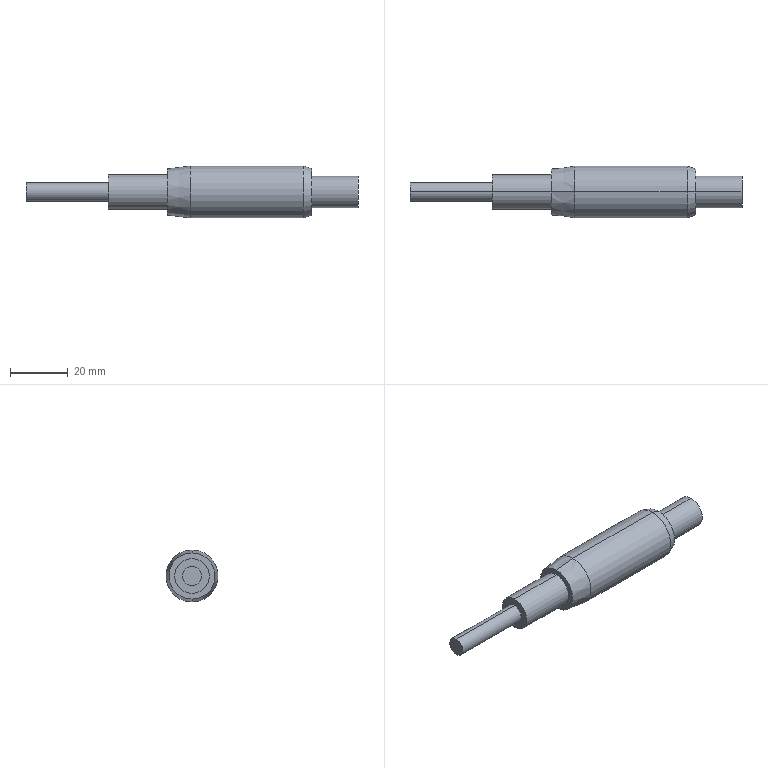Part | SolidWorks | features Revolution 1 | 1 solid | 17 faces | box 115 x 18 x 18 mm | volume 17209 mm3 | cylinder 8 | plane 5 | cone 4 | commonest cylinder face diameters 6.5 x2 11 x2 12 x2 18 x2
STEP:
#1=CARTESIAN_POINT('',(0.,0.,-3.25));
#2=VERTEX_POINT('',#1);
#3=CARTESIAN_POINT('',(0.,0.,3.25));
#4=VERTEX_POINT('',#3);
#5=CARTESIAN_POINT('',(0.,0.,0.));
#6=DIRECTION('',(1.,0.,0.));
#7=DIRECTION('',(0.,0.,-1.));
#8=AXIS2_PLACEMENT_3D('',#5,#6,#7);
#9=CIRCLE('',#8,3.25);
#10=EDGE_CURVE('',#2,#4,#9,.T.);
#11=ORIENTED_EDGE('',*,*,#10,.T.);
#12=CARTESIAN_POINT('',(28.5,0.,3.25));
#13=VERTEX_POINT('',#12);
#14=CARTESIAN_POINT('',(115.,0.,3.25));
#15=DIRECTION('',(1.,0.,0.));
#16=VECTOR('',#15,1000.);
#17=LINE('',#14,#16);
#18=EDGE_CURVE('',#4,#13,#17,.T.);
#19=ORIENTED_EDGE('',*,*,#18,.T.);
#20=CARTESIAN_POINT('',(28.5,0.,-3.25));
#21=VERTEX_POINT('',#20);
#22=CARTESIAN_POINT('',(28.5,0.,0.));
#23=DIRECTION('',(1.,0.,0.));
#24=DIRECTION('',(0.,0.,-1.));
#25=AXIS2_PLACEMENT_3D('',#22,#23,#24);
#26=CIRCLE('',#25,3.25);
#27=EDGE_CURVE('',#21,#13,#26,.T.);
#28=ORIENTED_EDGE('',*,*,#27,.F.);
#29=CARTESIAN_POINT('',(115.,0.,-3.25));
#30=DIRECTION('',(1.,0.,0.));
#31=VECTOR('',#30,1000.);
#32=LINE('',#29,#31);
#33=EDGE_CURVE('',#2,#21,#32,.T.);
#34=ORIENTED_EDGE('',*,*,#33,.F.);
#35=EDGE_LOOP('',(#11,#19,#28,#34));
#36=FACE_OUTER_BOUND('',#35,.T.);
#37=CARTESIAN_POINT('',(115.,0.,0.));
#38=DIRECTION('',(1.,0.,0.));
#39=DIRECTION('',(0.,0.,-1.));
#40=AXIS2_PLACEMENT_3D('',#37,#38,#39);
#41=CYLINDRICAL_SURFACE('',#40,3.25);
#42=ADVANCED_FACE('',(#36),#41,.T.);
#43=CARTESIAN_POINT('',(99.,0.,-5.5));
#44=VERTEX_POINT('',#43);
#45=CARTESIAN_POINT('',(99.,0.,5.5));
#46=VERTEX_POINT('',#45);
#47=CARTESIAN_POINT('',(99.,0.,0.));
#48=DIRECTION('',(1.,0.,0.));
#49=DIRECTION('',(0.,0.,-1.));
#50=AXIS2_PLACEMENT_3D('',#47,#48,#49);
#51=CIRCLE('',#50,5.5);
#52=EDGE_CURVE('',#44,#46,#51,.T.);
#53=ORIENTED_EDGE('',*,*,#52,.T.);
#54=CARTESIAN_POINT('',(115.,0.,5.5));
#55=VERTEX_POINT('',#54);
#56=CARTESIAN_POINT('',(115.,0.,5.5));
#57=DIRECTION('',(1.,0.,0.));
#58=VECTOR('',#57,1000.);
#59=LINE('',#56,#58);
#60=EDGE_CURVE('',#46,#55,#59,.T.);
#61=ORIENTED_EDGE('',*,*,#60,.T.);
#62=CARTESIAN_POINT('',(115.,0.,-5.5));
#63=VERTEX_POINT('',#62);
#64=CARTESIAN_POINT('',(115.,0.,0.));
#65=DIRECTION('',(1.,0.,0.));
#66=DIRECTION('',(0.,0.,-1.));
#67=AXIS2_PLACEMENT_3D('',#64,#65,#66);
#68=CIRCLE('',#67,5.5);
#69=EDGE_CURVE('',#63,#55,#68,.T.);
#70=ORIENTED_EDGE('',*,*,#69,.F.);
#71=CARTESIAN_POINT('',(115.,0.,-5.5));
#72=DIRECTION('',(1.,0.,0.));
#73=VECTOR('',#72,1000.);
#74=LINE('',#71,#73);
#75=EDGE_CURVE('',#44,#63,#74,.T.);
#76=ORIENTED_EDGE('',*,*,#75,.F.);
#77=EDGE_LOOP('',(#53,#61,#70,#76));
#78=FACE_OUTER_BOUND('',#77,.T.);
#79=CARTESIAN_POINT('',(115.,0.,0.));
#80=DIRECTION('',(1.,0.,0.));
#81=DIRECTION('',(0.,0.,-1.));
#82=AXIS2_PLACEMENT_3D('',#79,#80,#81);
#83=CYLINDRICAL_SURFACE('',#82,5.5);
#84=ADVANCED_FACE('',(#78),#83,.T.);
#85=CARTESIAN_POINT('',(99.,0.,-8.));
#86=VERTEX_POINT('',#85);
#87=CARTESIAN_POINT('',(99.,0.,8.));
#88=VERTEX_POINT('',#87);
#89=CARTESIAN_POINT('',(99.,0.,0.));
#90=DIRECTION('',(1.,0.,0.));
#91=DIRECTION('',(0.,0.,-1.));
#92=AXIS2_PLACEMENT_3D('',#89,#90,#91);
#93=CIRCLE('',#92,8.);
#94=EDGE_CURVE('',#86,#88,#93,.T.);
#95=ORIENTED_EDGE('',*,*,#94,.F.);
#96=CARTESIAN_POINT('',(96.,0.,-9.));
#97=VERTEX_POINT('',#96);
#98=CARTESIAN_POINT('',(99.,0.,-8.));
#99=DIRECTION('',(-0.9487,0.,-0.3162));
#100=VECTOR('',#99,1000.);
#101=LINE('',#98,#100);
#102=EDGE_CURVE('',#86,#97,#101,.T.);
#103=ORIENTED_EDGE('',*,*,#102,.T.);
#104=CARTESIAN_POINT('',(96.,0.,9.));
#105=VERTEX_POINT('',#104);
#106=CARTESIAN_POINT('',(96.,0.,0.));
#107=DIRECTION('',(1.,0.,0.));
#108=DIRECTION('',(0.,0.,-1.));
#109=AXIS2_PLACEMENT_3D('',#106,#107,#108);
#110=CIRCLE('',#109,9.);
#111=EDGE_CURVE('',#97,#105,#110,.T.);
#112=ORIENTED_EDGE('',*,*,#111,.T.);
#113=CARTESIAN_POINT('',(99.,0.,8.));
#114=DIRECTION('',(-0.9487,0.,0.3162));
#115=VECTOR('',#114,1000.);
#116=LINE('',#113,#115);
#117=EDGE_CURVE('',#88,#105,#116,.T.);
#118=ORIENTED_EDGE('',*,*,#117,.F.);
#119=EDGE_LOOP('',(#95,#103,#112,#118));
#120=FACE_OUTER_BOUND('',#119,.T.);
#121=CARTESIAN_POINT('',(99.,0.,0.));
#122=DIRECTION('',(-1.,0.,0.));
#123=DIRECTION('',(0.,0.,1.));
#124=AXIS2_PLACEMENT_3D('',#121,#122,#123);
#125=CONICAL_SURFACE('',#124,8.,0.3218);
#126=ADVANCED_FACE('',(#120),#125,.T.);
#127=CARTESIAN_POINT('',(57.,0.,-9.));
#128=VERTEX_POINT('',#127);
#129=CARTESIAN_POINT('',(57.,0.,9.));
#130=VERTEX_POINT('',#129);
#131=CARTESIAN_POINT('',(57.,0.,0.));
#132=DIRECTION('',(1.,0.,0.));
#133=DIRECTION('',(0.,0.,-1.));
#134=AXIS2_PLACEMENT_3D('',#131,#132,#133);
#135=CIRCLE('',#134,9.);
#136=EDGE_CURVE('',#128,#130,#135,.T.);
#137=ORIENTED_EDGE('',*,*,#136,.T.);
#138=CARTESIAN_POINT('',(115.,0.,9.));
#139=DIRECTION('',(1.,0.,0.));
#140=VECTOR('',#139,1000.);
#141=LINE('',#138,#140);
#142=EDGE_CURVE('',#130,#105,#141,.T.);
#143=ORIENTED_EDGE('',*,*,#142,.T.);
#144=ORIENTED_EDGE('',*,*,#111,.F.);
#145=CARTESIAN_POINT('',(115.,0.,-9.));
#146=DIRECTION('',(1.,0.,0.));
#147=VECTOR('',#146,1000.);
#148=LINE('',#145,#147);
#149=EDGE_CURVE('',#128,#97,#148,.T.);
#150=ORIENTED_EDGE('',*,*,#149,.F.);
#151=EDGE_LOOP('',(#137,#143,#144,#150));
#152=FACE_OUTER_BOUND('',#151,.T.);
#153=CARTESIAN_POINT('',(115.,0.,0.));
#154=DIRECTION('',(1.,0.,0.));
#155=DIRECTION('',(0.,0.,-1.));
#156=AXIS2_PLACEMENT_3D('',#153,#154,#155);
#157=CYLINDRICAL_SURFACE('',#156,9.);
#158=ADVANCED_FACE('',(#152),#157,.T.);
#159=CARTESIAN_POINT('',(49.,0.,-8.));
#160=VERTEX_POINT('',#159);
#161=CARTESIAN_POINT('',(49.,0.,8.));
#162=VERTEX_POINT('',#161);
#163=CARTESIAN_POINT('',(49.,0.,0.));
#164=DIRECTION('',(1.,0.,0.));
#165=DIRECTION('',(0.,0.,-1.));
#166=AXIS2_PLACEMENT_3D('',#163,#164,#165);
#167=CIRCLE('',#166,8.);
#168=EDGE_CURVE('',#160,#162,#167,.T.);
#169=ORIENTED_EDGE('',*,*,#168,.T.);
#170=CARTESIAN_POINT('',(57.,0.,9.));
#171=DIRECTION('',(0.9923,0.,0.124));
#172=VECTOR('',#171,1000.);
#173=LINE('',#170,#172);
#174=EDGE_CURVE('',#162,#130,#173,.T.);
#175=ORIENTED_EDGE('',*,*,#174,.T.);
#176=ORIENTED_EDGE('',*,*,#136,.F.);
#177=CARTESIAN_POINT('',(57.,0.,-9.));
#178=DIRECTION('',(0.9923,0.,-0.124));
#179=VECTOR('',#178,1000.);
#180=LINE('',#177,#179);
#181=EDGE_CURVE('',#160,#128,#180,.T.);
#182=ORIENTED_EDGE('',*,*,#181,.F.);
#183=EDGE_LOOP('',(#169,#175,#176,#182));
#184=FACE_OUTER_BOUND('',#183,.T.);
#185=CARTESIAN_POINT('',(57.,0.,0.));
#186=DIRECTION('',(1.,0.,0.));
#187=DIRECTION('',(0.,0.,-1.));
#188=AXIS2_PLACEMENT_3D('',#185,#186,#187);
#189=CONICAL_SURFACE('',#188,9.,0.1244);
#190=ADVANCED_FACE('',(#184),#189,.T.);
#191=CARTESIAN_POINT('',(28.5,0.,-6.));
#192=VERTEX_POINT('',#191);
#193=CARTESIAN_POINT('',(28.5,0.,6.));
#194=VERTEX_POINT('',#193);
#195=CARTESIAN_POINT('',(28.5,0.,0.));
#196=DIRECTION('',(1.,0.,0.));
#197=DIRECTION('',(0.,0.,-1.));
#198=AXIS2_PLACEMENT_3D('',#195,#196,#197);
#199=CIRCLE('',#198,6.);
#200=EDGE_CURVE('',#192,#194,#199,.T.);
#201=ORIENTED_EDGE('',*,*,#200,.T.);
#202=CARTESIAN_POINT('',(49.,0.,6.));
#203=VERTEX_POINT('',#202);
#204=CARTESIAN_POINT('',(115.,0.,6.));
#205=DIRECTION('',(1.,0.,0.));
#206=VECTOR('',#205,1000.);
#207=LINE('',#204,#206);
#208=EDGE_CURVE('',#194,#203,#207,.T.);
#209=ORIENTED_EDGE('',*,*,#208,.T.);
#210=CARTESIAN_POINT('',(49.,0.,-6.));
#211=VERTEX_POINT('',#210);
#212=CARTESIAN_POINT('',(49.,0.,0.));
#213=DIRECTION('',(1.,0.,0.));
#214=DIRECTION('',(0.,0.,-1.));
#215=AXIS2_PLACEMENT_3D('',#212,#213,#214);
#216=CIRCLE('',#215,6.);
#217=EDGE_CURVE('',#211,#203,#216,.T.);
#218=ORIENTED_EDGE('',*,*,#217,.F.);
#219=CARTESIAN_POINT('',(115.,0.,-6.));
#220=DIRECTION('',(1.,0.,0.));
#221=VECTOR('',#220,1000.);
#222=LINE('',#219,#221);
#223=EDGE_CURVE('',#192,#211,#222,.T.);
#224=ORIENTED_EDGE('',*,*,#223,.F.);
#225=EDGE_LOOP('',(#201,#209,#218,#224));
#226=FACE_OUTER_BOUND('',#225,.T.);
#227=CARTESIAN_POINT('',(115.,0.,0.));
#228=DIRECTION('',(1.,0.,0.));
#229=DIRECTION('',(0.,0.,-1.));
#230=AXIS2_PLACEMENT_3D('',#227,#228,#229);
#231=CYLINDRICAL_SURFACE('',#230,6.);
#232=ADVANCED_FACE('',(#226),#231,.T.);
#233=ORIENTED_EDGE('',*,*,#27,.T.);
#234=CARTESIAN_POINT('',(28.5,0.,0.));
#235=DIRECTION('',(1.,0.,0.));
#236=DIRECTION('',(0.,0.,-1.));
#237=AXIS2_PLACEMENT_3D('',#234,#235,#236);
#238=CIRCLE('',#237,3.25);
#239=EDGE_CURVE('',#13,#21,#238,.T.);
#240=ORIENTED_EDGE('',*,*,#239,.T.);
#241=EDGE_LOOP('',(#233,#240));
#242=FACE_BOUND('',#241,.T.);
#243=ORIENTED_EDGE('',*,*,#200,.F.);
#244=CARTESIAN_POINT('',(28.5,0.,0.));
#245=DIRECTION('',(1.,0.,0.));
#246=DIRECTION('',(0.,0.,-1.));
#247=AXIS2_PLACEMENT_3D('',#244,#245,#246);
#248=CIRCLE('',#247,6.);
#249=EDGE_CURVE('',#194,#192,#248,.T.);
#250=ORIENTED_EDGE('',*,*,#249,.F.);
#251=EDGE_LOOP('',(#243,#250));
#252=FACE_OUTER_BOUND('',#251,.T.);
#253=CARTESIAN_POINT('',(28.5,6.,0.));
#254=DIRECTION('',(-1.,0.,0.));
#255=DIRECTION('',(0.,0.,1.));
#256=AXIS2_PLACEMENT_3D('',#253,#254,#255);
#257=PLANE('',#256);
#258=ADVANCED_FACE('',(#242,#252),#257,.T.);
#259=ORIENTED_EDGE('',*,*,#208,.F.);
#260=ORIENTED_EDGE('',*,*,#249,.T.);
#261=ORIENTED_EDGE('',*,*,#223,.T.);
#262=CARTESIAN_POINT('',(49.,0.,0.));
#263=DIRECTION('',(1.,0.,0.));
#264=DIRECTION('',(0.,0.,-1.));
#265=AXIS2_PLACEMENT_3D('',#262,#263,#264);
#266=CIRCLE('',#265,6.);
#267=EDGE_CURVE('',#203,#211,#266,.T.);
#268=ORIENTED_EDGE('',*,*,#267,.F.);
#269=EDGE_LOOP('',(#259,#260,#261,#268));
#270=FACE_OUTER_BOUND('',#269,.T.);
#271=CARTESIAN_POINT('',(115.,0.,0.));
#272=DIRECTION('',(1.,0.,0.));
#273=DIRECTION('',(0.,0.,-1.));
#274=AXIS2_PLACEMENT_3D('',#271,#272,#273);
#275=CYLINDRICAL_SURFACE('',#274,6.);
#276=ADVANCED_FACE('',(#270),#275,.T.);
#277=ORIENTED_EDGE('',*,*,#217,.T.);
#278=ORIENTED_EDGE('',*,*,#267,.T.);
#279=EDGE_LOOP('',(#277,#278));
#280=FACE_BOUND('',#279,.T.);
#281=ORIENTED_EDGE('',*,*,#168,.F.);
#282=CARTESIAN_POINT('',(49.,0.,0.));
#283=DIRECTION('',(1.,0.,0.));
#284=DIRECTION('',(0.,0.,-1.));
#285=AXIS2_PLACEMENT_3D('',#282,#283,#284);
#286=CIRCLE('',#285,8.);
#287=EDGE_CURVE('',#162,#160,#286,.T.);
#288=ORIENTED_EDGE('',*,*,#287,.F.);
#289=EDGE_LOOP('',(#281,#288));
#290=FACE_OUTER_BOUND('',#289,.T.);
#291=CARTESIAN_POINT('',(49.,8.,0.));
#292=DIRECTION('',(-1.,0.,0.));
#293=DIRECTION('',(0.,0.,1.));
#294=AXIS2_PLACEMENT_3D('',#291,#292,#293);
#295=PLANE('',#294);
#296=ADVANCED_FACE('',(#280,#290),#295,.T.);
#297=ORIENTED_EDGE('',*,*,#174,.F.);
#298=ORIENTED_EDGE('',*,*,#287,.T.);
#299=ORIENTED_EDGE('',*,*,#181,.T.);
#300=CARTESIAN_POINT('',(57.,0.,0.));
#301=DIRECTION('',(1.,0.,0.));
#302=DIRECTION('',(0.,0.,-1.));
#303=AXIS2_PLACEMENT_3D('',#300,#301,#302);
#304=CIRCLE('',#303,9.);
#305=EDGE_CURVE('',#130,#128,#304,.T.);
#306=ORIENTED_EDGE('',*,*,#305,.F.);
#307=EDGE_LOOP('',(#297,#298,#299,#306));
#308=FACE_OUTER_BOUND('',#307,.T.);
#309=CARTESIAN_POINT('',(57.,0.,0.));
#310=DIRECTION('',(1.,0.,0.));
#311=DIRECTION('',(0.,0.,-1.));
#312=AXIS2_PLACEMENT_3D('',#309,#310,#311);
#313=CONICAL_SURFACE('',#312,9.,0.1244);
#314=ADVANCED_FACE('',(#308),#313,.T.);
#315=ORIENTED_EDGE('',*,*,#142,.F.);
#316=ORIENTED_EDGE('',*,*,#305,.T.);
#317=ORIENTED_EDGE('',*,*,#149,.T.);
#318=CARTESIAN_POINT('',(96.,0.,0.));
#319=DIRECTION('',(1.,0.,0.));
#320=DIRECTION('',(0.,0.,-1.));
#321=AXIS2_PLACEMENT_3D('',#318,#319,#320);
#322=CIRCLE('',#321,9.);
#323=EDGE_CURVE('',#105,#97,#322,.T.);
#324=ORIENTED_EDGE('',*,*,#323,.F.);
#325=EDGE_LOOP('',(#315,#316,#317,#324));
#326=FACE_OUTER_BOUND('',#325,.T.);
#327=CARTESIAN_POINT('',(115.,0.,0.));
#328=DIRECTION('',(1.,0.,0.));
#329=DIRECTION('',(0.,0.,-1.));
#330=AXIS2_PLACEMENT_3D('',#327,#328,#329);
#331=CYLINDRICAL_SURFACE('',#330,9.);
#332=ADVANCED_FACE('',(#326),#331,.T.);
#333=ORIENTED_EDGE('',*,*,#102,.F.);
#334=CARTESIAN_POINT('',(99.,0.,0.));
#335=DIRECTION('',(1.,0.,0.));
#336=DIRECTION('',(0.,0.,-1.));
#337=AXIS2_PLACEMENT_3D('',#334,#335,#336);
#338=CIRCLE('',#337,8.);
#339=EDGE_CURVE('',#88,#86,#338,.T.);
#340=ORIENTED_EDGE('',*,*,#339,.F.);
#341=ORIENTED_EDGE('',*,*,#117,.T.);
#342=ORIENTED_EDGE('',*,*,#323,.T.);
#343=EDGE_LOOP('',(#333,#340,#341,#342));
#344=FACE_OUTER_BOUND('',#343,.T.);
#345=CARTESIAN_POINT('',(99.,0.,0.));
#346=DIRECTION('',(-1.,0.,0.));
#347=DIRECTION('',(0.,0.,1.));
#348=AXIS2_PLACEMENT_3D('',#345,#346,#347);
#349=CONICAL_SURFACE('',#348,8.,0.3218);
#350=ADVANCED_FACE('',(#344),#349,.T.);
#351=ORIENTED_EDGE('',*,*,#339,.T.);
#352=ORIENTED_EDGE('',*,*,#94,.T.);
#353=EDGE_LOOP('',(#351,#352));
#354=FACE_OUTER_BOUND('',#353,.T.);
#355=ORIENTED_EDGE('',*,*,#52,.F.);
#356=CARTESIAN_POINT('',(99.,0.,0.));
#357=DIRECTION('',(1.,0.,0.));
#358=DIRECTION('',(0.,0.,-1.));
#359=AXIS2_PLACEMENT_3D('',#356,#357,#358);
#360=CIRCLE('',#359,5.5);
#361=EDGE_CURVE('',#46,#44,#360,.T.);
#362=ORIENTED_EDGE('',*,*,#361,.F.);
#363=EDGE_LOOP('',(#355,#362));
#364=FACE_BOUND('',#363,.T.);
#365=CARTESIAN_POINT('',(99.,5.5,0.));
#366=DIRECTION('',(1.,0.,0.));
#367=DIRECTION('',(0.,0.,-1.));
#368=AXIS2_PLACEMENT_3D('',#365,#366,#367);
#369=PLANE('',#368);
#370=ADVANCED_FACE('',(#354,#364),#369,.T.);
#371=ORIENTED_EDGE('',*,*,#60,.F.);
#372=ORIENTED_EDGE('',*,*,#361,.T.);
#373=ORIENTED_EDGE('',*,*,#75,.T.);
#374=CARTESIAN_POINT('',(115.,0.,0.));
#375=DIRECTION('',(1.,0.,0.));
#376=DIRECTION('',(0.,0.,-1.));
#377=AXIS2_PLACEMENT_3D('',#374,#375,#376);
#378=CIRCLE('',#377,5.5);
#379=EDGE_CURVE('',#55,#63,#378,.T.);
#380=ORIENTED_EDGE('',*,*,#379,.F.);
#381=EDGE_LOOP('',(#371,#372,#373,#380));
#382=FACE_OUTER_BOUND('',#381,.T.);
#383=CARTESIAN_POINT('',(115.,0.,0.));
#384=DIRECTION('',(1.,0.,0.));
#385=DIRECTION('',(0.,0.,-1.));
#386=AXIS2_PLACEMENT_3D('',#383,#384,#385);
#387=CYLINDRICAL_SURFACE('',#386,5.5);
#388=ADVANCED_FACE('',(#382),#387,.T.);
#389=ORIENTED_EDGE('',*,*,#69,.T.);
#390=ORIENTED_EDGE('',*,*,#379,.T.);
#391=EDGE_LOOP('',(#389,#390));
#392=FACE_OUTER_BOUND('',#391,.T.);
#393=CARTESIAN_POINT('',(115.,0.,0.));
#394=DIRECTION('',(1.,0.,0.));
#395=DIRECTION('',(0.,0.,-1.));
#396=AXIS2_PLACEMENT_3D('',#393,#394,#395);
#397=PLANE('',#396);
#398=ADVANCED_FACE('',(#392),#397,.T.);
#399=ORIENTED_EDGE('',*,*,#10,.F.);
#400=CARTESIAN_POINT('',(0.,0.,0.));
#401=DIRECTION('',(1.,0.,0.));
#402=DIRECTION('',(0.,0.,-1.));
#403=AXIS2_PLACEMENT_3D('',#400,#401,#402);
#404=CIRCLE('',#403,3.25);
#405=EDGE_CURVE('',#4,#2,#404,.T.);
#406=ORIENTED_EDGE('',*,*,#405,.F.);
#407=EDGE_LOOP('',(#399,#406));
#408=FACE_OUTER_BOUND('',#407,.T.);
#409=CARTESIAN_POINT('',(0.,3.25,0.));
#410=DIRECTION('',(-1.,0.,0.));
#411=DIRECTION('',(0.,0.,1.));
#412=AXIS2_PLACEMENT_3D('',#409,#410,#411);
#413=PLANE('',#412);
#414=ADVANCED_FACE('',(#408),#413,.T.);
#415=ORIENTED_EDGE('',*,*,#18,.F.);
#416=ORIENTED_EDGE('',*,*,#405,.T.);
#417=ORIENTED_EDGE('',*,*,#33,.T.);
#418=ORIENTED_EDGE('',*,*,#239,.F.);
#419=EDGE_LOOP('',(#415,#416,#417,#418));
#420=FACE_OUTER_BOUND('',#419,.T.);
#421=CARTESIAN_POINT('',(115.,0.,0.));
#422=DIRECTION('',(1.,0.,0.));
#423=DIRECTION('',(0.,0.,-1.));
#424=AXIS2_PLACEMENT_3D('',#421,#422,#423);
#425=CYLINDRICAL_SURFACE('',#424,3.25);
#426=ADVANCED_FACE('',(#420),#425,.T.);
#427=CLOSED_SHELL('',(#42,#84,#126,#158,#190,#232,#258,#276,#296,#314,#332,#350,#370,#388,#398,#414,#426));
#428=MANIFOLD_SOLID_BREP('',#427);
#429=CARTESIAN_POINT('',(0.,0.,0.));
#430=DIRECTION('',(0.,0.,1.));
#431=DIRECTION('',(1.,0.,0.));
#432=AXIS2_PLACEMENT_3D('',#429,#430,#431);
#433=(LENGTH_UNIT()NAMED_UNIT(*)SI_UNIT(.MILLI.,.METRE.));
#434=UNCERTAINTY_MEASURE_WITH_UNIT(LENGTH_MEASURE(0.00001),#433,'','');
#435=(NAMED_UNIT(*)PLANE_ANGLE_UNIT()SI_UNIT($,.RADIAN.));
#436=(NAMED_UNIT(*)SI_UNIT($,.STERADIAN.)SOLID_ANGLE_UNIT());
#437=(GEOMETRIC_REPRESENTATION_CONTEXT(3)GLOBAL_UNCERTAINTY_ASSIGNED_CONTEXT((#434))GLOBAL_UNIT_ASSIGNED_CONTEXT((#433,#435,#436))REPRESENTATION_CONTEXT('',''));
#438=ADVANCED_BREP_SHAPE_REPRESENTATION('',(#428,#432),#437);